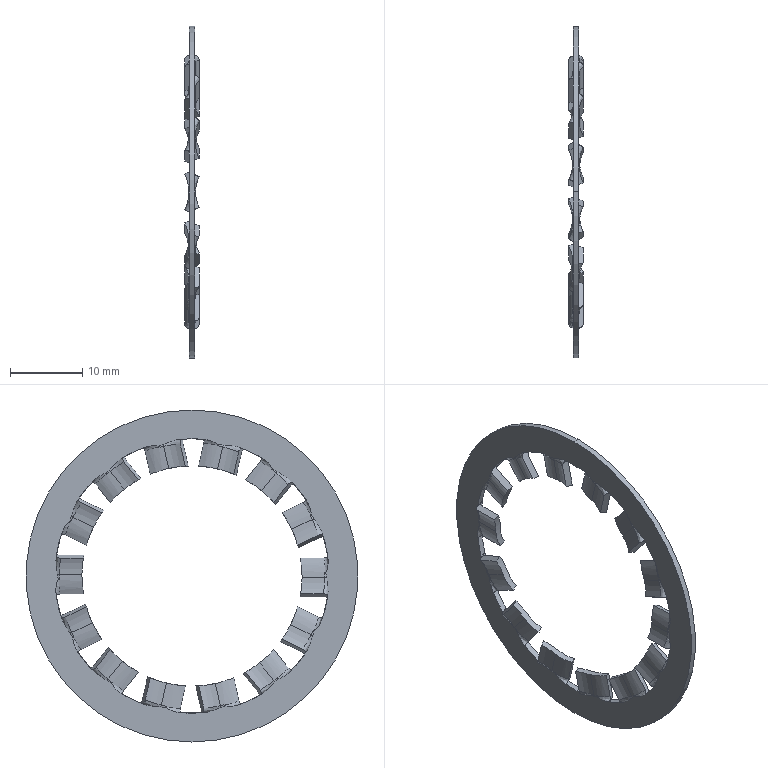Part | SolidWorks | features RefAxis 3, BaseBody 1 | 1 solid | 229 faces | box 2 x 46 x 46 mm | volume 665.952 mm3 | cylinder 115 | spline 84 | plane 30 | commonest cylinder face diameters 38 x43 11.374 x28 12.913 x14 12.974 x14 30.5 x14 46 x2